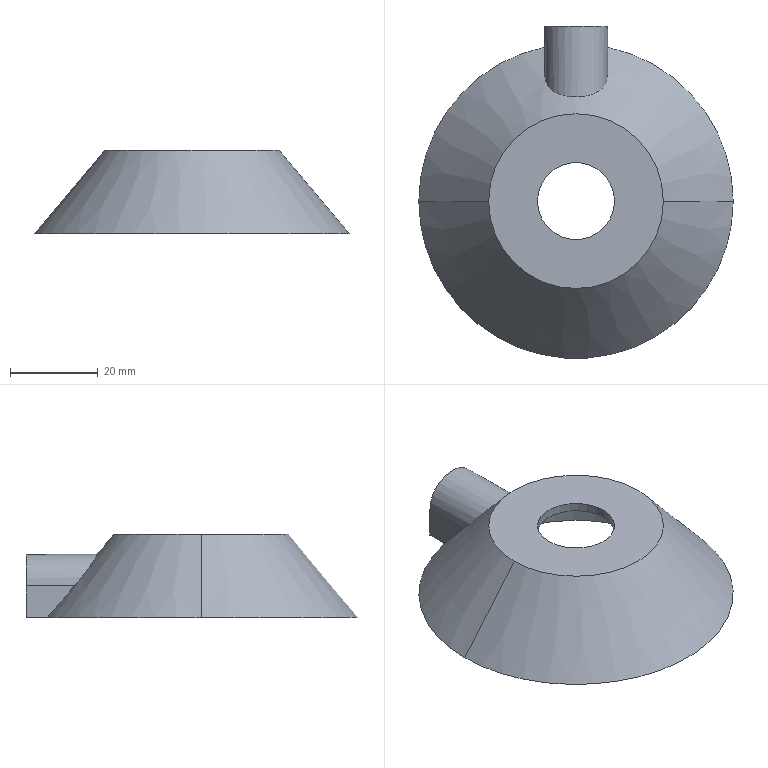Part | SolidWorks | features ICE 5, Extrusion 1, RevCut 1 | 1 solid | 30 faces | box 71.8 x 75.9 x 19 mm | volume 15603 mm3 | plane 12 | cylinder 11 | cone 7 | commonest cylinder face diameters 58 x3 62 x3 5.4 x2 17.6 x2 14.4 x1
STEP:
#1=CARTESIAN_POINT('',(2.7,26.139,6.7));
#2=VERTEX_POINT('',#1);
#3=CARTESIAN_POINT('',(0.,24.012,9.4));
#4=VERTEX_POINT('',#3);
#5=CARTESIAN_POINT('',(2.7,26.139,6.7));
#6=CARTESIAN_POINT('',(2.7,26.009,6.854));
#7=CARTESIAN_POINT('',(2.687,25.881,7.008));
#8=CARTESIAN_POINT('',(2.633,25.626,7.316));
#9=CARTESIAN_POINT('',(2.593,25.5,7.471));
#10=CARTESIAN_POINT('',(2.483,25.256,7.773));
#11=CARTESIAN_POINT('',(2.414,25.138,7.921));
#12=CARTESIAN_POINT('',(2.246,24.912,8.208));
#13=CARTESIAN_POINT('',(2.145,24.802,8.349));
#14=CARTESIAN_POINT('',(1.914,24.599,8.612));
#15=CARTESIAN_POINT('',(1.784,24.506,8.735));
#16=CARTESIAN_POINT('',(1.492,24.338,8.958));
#17=CARTESIAN_POINT('',(1.329,24.264,9.058));
#18=CARTESIAN_POINT('',(0.9814,24.142,9.223));
#19=CARTESIAN_POINT('',(0.7923,24.094,9.289));
#20=CARTESIAN_POINT('',(0.4032,24.029,9.377));
#21=CARTESIAN_POINT('',(0.204,24.012,9.4));
#22=CARTESIAN_POINT('',(0.,24.012,9.4));
#23=B_SPLINE_CURVE_WITH_KNOTS('',3,(#5,#6,#7,#8,#9,#10,#11,#12,#13,#14,#15,#16,#17,#18,#19,#20,#21,#22),.UNSPECIFIED.,.F.,.F.,(4,2,2,2,2,2,2,2,4),(0.0003524,0.0009553,0.001558,0.002161,0.002764,0.003367,0.00397,0.004572,0.005175),.UNSPECIFIED.);
#24=EDGE_CURVE('',#2,#4,#23,.T.);
#25=ORIENTED_EDGE('',*,*,#24,.T.);
#26=CARTESIAN_POINT('',(0.,40.,9.4));
#27=VERTEX_POINT('',#26);
#28=CARTESIAN_POINT('',(0.,24.,9.4));
#29=DIRECTION('',(0.,1.,0.));
#30=VECTOR('',#29,1000.);
#31=LINE('',#28,#30);
#32=EDGE_CURVE('',#4,#27,#31,.T.);
#33=ORIENTED_EDGE('',*,*,#32,.T.);
#34=CARTESIAN_POINT('',(2.7,40.,6.7));
#35=VERTEX_POINT('',#34);
#36=CARTESIAN_POINT('',(0.,40.,6.7));
#37=DIRECTION('',(0.,1.,0.));
#38=DIRECTION('',(0.,0.,1.));
#39=AXIS2_PLACEMENT_3D('',#36,#37,#38);
#40=CIRCLE('',#39,2.7);
#41=EDGE_CURVE('',#27,#35,#40,.T.);
#42=ORIENTED_EDGE('',*,*,#41,.T.);
#43=CARTESIAN_POINT('',(2.7,24.,6.7));
#44=DIRECTION('',(0.,1.,0.));
#45=VECTOR('',#44,1000.);
#46=LINE('',#43,#45);
#47=EDGE_CURVE('',#2,#35,#46,.T.);
#48=ORIENTED_EDGE('',*,*,#47,.F.);
#49=EDGE_LOOP('',(#25,#33,#42,#48));
#50=FACE_OUTER_BOUND('',#49,.T.);
#51=CARTESIAN_POINT('',(0.,24.,6.7));
#52=DIRECTION('',(0.,1.,0.));
#53=DIRECTION('',(0.,0.,1.));
#54=AXIS2_PLACEMENT_3D('',#51,#52,#53);
#55=CYLINDRICAL_SURFACE('',#54,2.7);
#56=ADVANCED_FACE('',(#50),#55,.F.);
#57=CARTESIAN_POINT('',(-8.8,0.,17.));
#58=VERTEX_POINT('',#57);
#59=CARTESIAN_POINT('',(8.8,0.,17.));
#60=VERTEX_POINT('',#59);
#61=CARTESIAN_POINT('',(0.,0.,17.));
#62=DIRECTION('',(0.,0.,1.));
#63=DIRECTION('',(1.,0.,0.));
#64=AXIS2_PLACEMENT_3D('',#61,#62,#63);
#65=CIRCLE('',#64,8.8);
#66=EDGE_CURVE('',#58,#60,#65,.T.);
#67=ORIENTED_EDGE('',*,*,#66,.F.);
#68=CARTESIAN_POINT('',(-8.8,0.,19.));
#69=VERTEX_POINT('',#68);
#70=CARTESIAN_POINT('',(-8.8,0.,17.));
#71=DIRECTION('',(0.,0.,1.));
#72=VECTOR('',#71,1000.);
#73=LINE('',#70,#72);
#74=EDGE_CURVE('',#58,#69,#73,.T.);
#75=ORIENTED_EDGE('',*,*,#74,.T.);
#76=CARTESIAN_POINT('',(8.8,0.,19.));
#77=VERTEX_POINT('',#76);
#78=CARTESIAN_POINT('',(0.,0.,19.));
#79=DIRECTION('',(0.,0.,1.));
#80=DIRECTION('',(1.,0.,0.));
#81=AXIS2_PLACEMENT_3D('',#78,#79,#80);
#82=CIRCLE('',#81,8.8);
#83=EDGE_CURVE('',#69,#77,#82,.T.);
#84=ORIENTED_EDGE('',*,*,#83,.T.);
#85=CARTESIAN_POINT('',(8.8,0.,17.));
#86=DIRECTION('',(0.,0.,1.));
#87=VECTOR('',#86,1000.);
#88=LINE('',#85,#87);
#89=EDGE_CURVE('',#60,#77,#88,.T.);
#90=ORIENTED_EDGE('',*,*,#89,.F.);
#91=EDGE_LOOP('',(#67,#75,#84,#90));
#92=FACE_OUTER_BOUND('',#91,.T.);
#93=CARTESIAN_POINT('',(0.,0.,17.));
#94=DIRECTION('',(0.,0.,1.));
#95=DIRECTION('',(1.,0.,0.));
#96=AXIS2_PLACEMENT_3D('',#93,#94,#95);
#97=CYLINDRICAL_SURFACE('',#96,8.8);
#98=ADVANCED_FACE('',(#92),#97,.F.);
#99=CARTESIAN_POINT('',(17.635,0.,17.));
#100=VERTEX_POINT('',#99);
#101=CARTESIAN_POINT('',(-17.635,0.,17.));
#102=VERTEX_POINT('',#101);
#103=CARTESIAN_POINT('',(0.,0.,17.));
#104=DIRECTION('',(0.,0.,-1.));
#105=DIRECTION('',(-1.,0.,0.));
#106=AXIS2_PLACEMENT_3D('',#103,#104,#105);
#107=CIRCLE('',#106,17.635);
#108=EDGE_CURVE('',#100,#102,#107,.T.);
#109=ORIENTED_EDGE('',*,*,#108,.F.);
#110=CARTESIAN_POINT('',(29.,0.,3.456));
#111=VERTEX_POINT('',#110);
#112=CARTESIAN_POINT('',(17.635,0.,17.));
#113=DIRECTION('',(0.6428,0.,-0.766));
#114=VECTOR('',#113,1000.);
#115=LINE('',#112,#114);
#116=EDGE_CURVE('',#100,#111,#115,.T.);
#117=ORIENTED_EDGE('',*,*,#116,.T.);
#118=CARTESIAN_POINT('',(-29.,0.,3.456));
#119=VERTEX_POINT('',#118);
#120=CARTESIAN_POINT('',(0.,0.,3.456));
#121=DIRECTION('',(0.,0.,1.));
#122=DIRECTION('',(-1.,0.,0.));
#123=AXIS2_PLACEMENT_3D('',#120,#121,#122);
#124=CIRCLE('',#123,29.);
#125=EDGE_CURVE('',#119,#111,#124,.T.);
#126=ORIENTED_EDGE('',*,*,#125,.F.);
#127=CARTESIAN_POINT('',(-17.635,0.,17.));
#128=DIRECTION('',(-0.6428,0.,-0.766));
#129=VECTOR('',#128,1000.);
#130=LINE('',#127,#129);
#131=EDGE_CURVE('',#102,#119,#130,.T.);
#132=ORIENTED_EDGE('',*,*,#131,.F.);
#133=EDGE_LOOP('',(#109,#117,#126,#132));
#134=FACE_OUTER_BOUND('',#133,.T.);
#135=CARTESIAN_POINT('',(0.,0.,17.));
#136=DIRECTION('',(0.,0.,-1.));
#137=DIRECTION('',(-1.,0.,0.));
#138=AXIS2_PLACEMENT_3D('',#135,#136,#137);
#139=CONICAL_SURFACE('',#138,17.635,0.6981);
#140=ADVANCED_FACE('',(#134),#139,.F.);
#141=ORIENTED_EDGE('',*,*,#125,.T.);
#142=CARTESIAN_POINT('',(29.,0.,0.));
#143=VERTEX_POINT('',#142);
#144=CARTESIAN_POINT('',(29.,0.,38.017));
#145=DIRECTION('',(0.,0.,-1.));
#146=VECTOR('',#145,1000.);
#147=LINE('',#144,#146);
#148=EDGE_CURVE('',#111,#143,#147,.T.);
#149=ORIENTED_EDGE('',*,*,#148,.T.);
#150=CARTESIAN_POINT('',(-29.,0.,0.));
#151=VERTEX_POINT('',#150);
#152=CARTESIAN_POINT('',(0.,0.,0.));
#153=DIRECTION('',(0.,0.,-1.));
#154=DIRECTION('',(-1.,0.,0.));
#155=AXIS2_PLACEMENT_3D('',#152,#153,#154);
#156=CIRCLE('',#155,29.);
#157=EDGE_CURVE('',#143,#151,#156,.T.);
#158=ORIENTED_EDGE('',*,*,#157,.T.);
#159=CARTESIAN_POINT('',(-29.,0.,38.017));
#160=DIRECTION('',(0.,0.,-1.));
#161=VECTOR('',#160,1000.);
#162=LINE('',#159,#161);
#163=EDGE_CURVE('',#119,#151,#162,.T.);
#164=ORIENTED_EDGE('',*,*,#163,.F.);
#165=EDGE_LOOP('',(#141,#149,#158,#164));
#166=FACE_OUTER_BOUND('',#165,.T.);
#167=CARTESIAN_POINT('',(0.,0.,38.017));
#168=DIRECTION('',(0.,0.,-1.));
#169=DIRECTION('',(-1.,0.,0.));
#170=AXIS2_PLACEMENT_3D('',#167,#168,#169);
#171=CYLINDRICAL_SURFACE('',#170,29.);
#172=ADVANCED_FACE('',(#166),#171,.F.);
#173=CARTESIAN_POINT('',(-3.7,28.763,3.456));
#174=VERTEX_POINT('',#173);
#175=CARTESIAN_POINT('',(0.,0.,3.456));
#176=DIRECTION('',(0.,0.,1.));
#177=DIRECTION('',(-1.,0.,0.));
#178=AXIS2_PLACEMENT_3D('',#175,#176,#177);
#179=CIRCLE('',#178,29.);
#180=EDGE_CURVE('',#174,#119,#179,.T.);
#181=ORIENTED_EDGE('',*,*,#180,.T.);
#182=ORIENTED_EDGE('',*,*,#163,.T.);
#183=CARTESIAN_POINT('',(-3.7,28.763,0.));
#184=VERTEX_POINT('',#183);
#185=CARTESIAN_POINT('',(0.,0.,0.));
#186=DIRECTION('',(0.,0.,-1.));
#187=DIRECTION('',(-1.,0.,0.));
#188=AXIS2_PLACEMENT_3D('',#185,#186,#187);
#189=CIRCLE('',#188,29.);
#190=EDGE_CURVE('',#151,#184,#189,.T.);
#191=ORIENTED_EDGE('',*,*,#190,.T.);
#192=CARTESIAN_POINT('',(-3.7,28.763,38.017));
#193=DIRECTION('',(0.,0.,1.));
#194=VECTOR('',#193,1000.);
#195=LINE('',#192,#194);
#196=EDGE_CURVE('',#184,#174,#195,.T.);
#197=ORIENTED_EDGE('',*,*,#196,.T.);
#198=EDGE_LOOP('',(#181,#182,#191,#197));
#199=FACE_OUTER_BOUND('',#198,.T.);
#200=CARTESIAN_POINT('',(0.,0.,38.017));
#201=DIRECTION('',(0.,0.,-1.));
#202=DIRECTION('',(-1.,0.,0.));
#203=AXIS2_PLACEMENT_3D('',#200,#201,#202);
#204=CYLINDRICAL_SURFACE('',#203,29.);
#205=ADVANCED_FACE('',(#199),#204,.F.);
#206=CARTESIAN_POINT('',(5.9,30.433,1.073));
#207=VERTEX_POINT('',#206);
#208=CARTESIAN_POINT('',(31.,0.,1.073));
#209=VERTEX_POINT('',#208);
#210=CARTESIAN_POINT('',(0.,0.,1.073));
#211=DIRECTION('',(0.,0.,-1.));
#212=DIRECTION('',(-1.,0.,0.));
#213=AXIS2_PLACEMENT_3D('',#210,#211,#212);
#214=CIRCLE('',#213,31.);
#215=EDGE_CURVE('',#207,#209,#214,.T.);
#216=ORIENTED_EDGE('',*,*,#215,.T.);
#217=CARTESIAN_POINT('',(31.,0.,0.));
#218=VERTEX_POINT('',#217);
#219=CARTESIAN_POINT('',(31.,0.,38.017));
#220=DIRECTION('',(0.,0.,-1.));
#221=VECTOR('',#220,1000.);
#222=LINE('',#219,#221);
#223=EDGE_CURVE('',#209,#218,#222,.T.);
#224=ORIENTED_EDGE('',*,*,#223,.T.);
#225=CARTESIAN_POINT('',(5.9,30.433,0.));
#226=VERTEX_POINT('',#225);
#227=CARTESIAN_POINT('',(0.,0.,0.));
#228=DIRECTION('',(0.,0.,-1.));
#229=DIRECTION('',(-1.,0.,0.));
#230=AXIS2_PLACEMENT_3D('',#227,#228,#229);
#231=CIRCLE('',#230,31.);
#232=EDGE_CURVE('',#226,#218,#231,.T.);
#233=ORIENTED_EDGE('',*,*,#232,.F.);
#234=CARTESIAN_POINT('',(5.9,30.433,38.017));
#235=DIRECTION('',(0.,0.,-1.));
#236=VECTOR('',#235,1000.);
#237=LINE('',#234,#236);
#238=EDGE_CURVE('',#207,#226,#237,.T.);
#239=ORIENTED_EDGE('',*,*,#238,.F.);
#240=EDGE_LOOP('',(#216,#224,#233,#239));
#241=FACE_OUTER_BOUND('',#240,.T.);
#242=CARTESIAN_POINT('',(0.,0.,38.017));
#243=DIRECTION('',(0.,0.,-1.));
#244=DIRECTION('',(-1.,0.,0.));
#245=AXIS2_PLACEMENT_3D('',#242,#243,#244);
#246=CYLINDRICAL_SURFACE('',#245,31.);
#247=ADVANCED_FACE('',(#241),#246,.T.);
#248=ORIENTED_EDGE('',*,*,#223,.F.);
#249=CARTESIAN_POINT('',(-31.,0.,1.073));
#250=VERTEX_POINT('',#249);
#251=CARTESIAN_POINT('',(0.,0.,1.073));
#252=DIRECTION('',(0.,0.,-1.));
#253=DIRECTION('',(-1.,0.,0.));
#254=AXIS2_PLACEMENT_3D('',#251,#252,#253);
#255=CIRCLE('',#254,31.);
#256=EDGE_CURVE('',#209,#250,#255,.T.);
#257=ORIENTED_EDGE('',*,*,#256,.T.);
#258=CARTESIAN_POINT('',(-31.,0.,0.));
#259=VERTEX_POINT('',#258);
#260=CARTESIAN_POINT('',(-31.,0.,38.017));
#261=DIRECTION('',(0.,0.,-1.));
#262=VECTOR('',#261,1000.);
#263=LINE('',#260,#262);
#264=EDGE_CURVE('',#250,#259,#263,.T.);
#265=ORIENTED_EDGE('',*,*,#264,.T.);
#266=CARTESIAN_POINT('',(0.,0.,0.));
#267=DIRECTION('',(0.,0.,-1.));
#268=DIRECTION('',(-1.,0.,0.));
#269=AXIS2_PLACEMENT_3D('',#266,#267,#268);
#270=CIRCLE('',#269,31.);
#271=EDGE_CURVE('',#218,#259,#270,.T.);
#272=ORIENTED_EDGE('',*,*,#271,.F.);
#273=EDGE_LOOP('',(#248,#257,#265,#272));
#274=FACE_OUTER_BOUND('',#273,.T.);
#275=CARTESIAN_POINT('',(0.,0.,38.017));
#276=DIRECTION('',(0.,0.,-1.));
#277=DIRECTION('',(-1.,0.,0.));
#278=AXIS2_PLACEMENT_3D('',#275,#276,#277);
#279=CYLINDRICAL_SURFACE('',#278,31.);
#280=ADVANCED_FACE('',(#274),#279,.T.);
#281=ORIENTED_EDGE('',*,*,#256,.F.);
#282=CARTESIAN_POINT('',(31.9,0.,0.));
#283=VERTEX_POINT('',#282);
#284=CARTESIAN_POINT('',(17.635,0.,17.));
#285=DIRECTION('',(0.6428,0.,-0.766));
#286=VECTOR('',#285,1000.);
#287=LINE('',#284,#286);
#288=EDGE_CURVE('',#209,#283,#287,.T.);
#289=ORIENTED_EDGE('',*,*,#288,.T.);
#290=CARTESIAN_POINT('',(-31.9,0.,0.));
#291=VERTEX_POINT('',#290);
#292=CARTESIAN_POINT('',(0.,0.,0.));
#293=DIRECTION('',(0.,0.,-1.));
#294=DIRECTION('',(-1.,0.,0.));
#295=AXIS2_PLACEMENT_3D('',#292,#293,#294);
#296=CIRCLE('',#295,31.9);
#297=EDGE_CURVE('',#283,#291,#296,.T.);
#298=ORIENTED_EDGE('',*,*,#297,.T.);
#299=CARTESIAN_POINT('',(-17.635,0.,17.));
#300=DIRECTION('',(-0.6428,0.,-0.766));
#301=VECTOR('',#300,1000.);
#302=LINE('',#299,#301);
#303=EDGE_CURVE('',#250,#291,#302,.T.);
#304=ORIENTED_EDGE('',*,*,#303,.F.);
#305=EDGE_LOOP('',(#281,#289,#298,#304));
#306=FACE_OUTER_BOUND('',#305,.T.);
#307=CARTESIAN_POINT('',(0.,0.,17.));
#308=DIRECTION('',(0.,0.,-1.));
#309=DIRECTION('',(-1.,0.,0.));
#310=AXIS2_PLACEMENT_3D('',#307,#308,#309);
#311=CONICAL_SURFACE('',#310,17.635,0.6981);
#312=ADVANCED_FACE('',(#306),#311,.F.);
#313=CARTESIAN_POINT('',(-5.9,30.433,1.073));
#314=VERTEX_POINT('',#313);
#315=CARTESIAN_POINT('',(0.,0.,1.073));
#316=DIRECTION('',(0.,0.,-1.));
#317=DIRECTION('',(-1.,0.,0.));
#318=AXIS2_PLACEMENT_3D('',#315,#316,#317);
#319=CIRCLE('',#318,31.);
#320=EDGE_CURVE('',#250,#314,#319,.T.);
#321=ORIENTED_EDGE('',*,*,#320,.F.);
#322=ORIENTED_EDGE('',*,*,#303,.T.);
#323=CARTESIAN_POINT('',(-5.9,31.35,0.));
#324=VERTEX_POINT('',#323);
#325=CARTESIAN_POINT('',(0.,0.,0.));
#326=DIRECTION('',(0.,0.,-1.));
#327=DIRECTION('',(-1.,0.,0.));
#328=AXIS2_PLACEMENT_3D('',#325,#326,#327);
#329=CIRCLE('',#328,31.9);
#330=EDGE_CURVE('',#291,#324,#329,.T.);
#331=ORIENTED_EDGE('',*,*,#330,.T.);
#332=CARTESIAN_POINT('',(-5.9,30.433,1.073));
#333=CARTESIAN_POINT('',(-5.9,30.739,0.7151));
#334=CARTESIAN_POINT('',(-5.9,31.044,0.3576));
#335=CARTESIAN_POINT('',(-5.9,31.35,0.));
#336=B_SPLINE_CURVE_WITH_KNOTS('',3,(#332,#333,#334,#335),.UNSPECIFIED.,.F.,.F.,(4,4),(0.006323,0.007734),.UNSPECIFIED.);
#337=EDGE_CURVE('',#314,#324,#336,.T.);
#338=ORIENTED_EDGE('',*,*,#337,.F.);
#339=EDGE_LOOP('',(#321,#322,#331,#338));
#340=FACE_OUTER_BOUND('',#339,.T.);
#341=CARTESIAN_POINT('',(0.,0.,17.));
#342=DIRECTION('',(0.,0.,-1.));
#343=DIRECTION('',(-1.,0.,0.));
#344=AXIS2_PLACEMENT_3D('',#341,#342,#343);
#345=CONICAL_SURFACE('',#344,17.635,0.6981);
#346=ADVANCED_FACE('',(#340),#345,.F.);
#347=CARTESIAN_POINT('',(-19.957,0.,19.));
#348=VERTEX_POINT('',#347);
#349=CARTESIAN_POINT('',(19.957,0.,19.));
#350=VERTEX_POINT('',#349);
#351=CARTESIAN_POINT('',(0.,0.,19.));
#352=DIRECTION('',(0.,0.,1.));
#353=DIRECTION('',(1.,0.,0.));
#354=AXIS2_PLACEMENT_3D('',#351,#352,#353);
#355=CIRCLE('',#354,19.957);
#356=EDGE_CURVE('',#348,#350,#355,.T.);
#357=ORIENTED_EDGE('',*,*,#356,.F.);
#358=CARTESIAN_POINT('',(-35.9,0.,0.));
#359=VERTEX_POINT('',#358);
#360=CARTESIAN_POINT('',(-35.9,0.,0.));
#361=DIRECTION('',(-0.6428,0.,-0.766));
#362=VECTOR('',#361,1000.);
#363=LINE('',#360,#362);
#364=EDGE_CURVE('',#348,#359,#363,.T.);
#365=ORIENTED_EDGE('',*,*,#364,.T.);
#366=CARTESIAN_POINT('',(35.9,0.,0.));
#367=VERTEX_POINT('',#366);
#368=CARTESIAN_POINT('',(0.,0.,0.));
#369=DIRECTION('',(0.,0.,1.));
#370=DIRECTION('',(1.,0.,0.));
#371=AXIS2_PLACEMENT_3D('',#368,#369,#370);
#372=CIRCLE('',#371,35.9);
#373=EDGE_CURVE('',#359,#367,#372,.T.);
#374=ORIENTED_EDGE('',*,*,#373,.T.);
#375=CARTESIAN_POINT('',(35.9,0.,0.));
#376=DIRECTION('',(0.6428,0.,-0.766));
#377=VECTOR('',#376,1000.);
#378=LINE('',#375,#377);
#379=EDGE_CURVE('',#350,#367,#378,.T.);
#380=ORIENTED_EDGE('',*,*,#379,.F.);
#381=EDGE_LOOP('',(#357,#365,#374,#380));
#382=FACE_OUTER_BOUND('',#381,.T.);
#383=CARTESIAN_POINT('',(0.,0.,0.));
#384=DIRECTION('',(0.,0.,-1.));
#385=DIRECTION('',(1.,0.,0.));
#386=AXIS2_PLACEMENT_3D('',#383,#384,#385);
#387=CONICAL_SURFACE('',#386,35.9,0.6981);
#388=ADVANCED_FACE('',(#382),#387,.T.);
#389=CARTESIAN_POINT('',(-5.9,30.433,0.));
#390=VERTEX_POINT('',#389);
#391=CARTESIAN_POINT('',(-5.9,-35.901,0.));
#392=DIRECTION('',(0.,1.,0.));
#393=VECTOR('',#392,1000.);
#394=LINE('',#391,#393);
#395=EDGE_CURVE('',#390,#324,#394,.T.);
#396=ORIENTED_EDGE('',*,*,#395,.T.);
#397=ORIENTED_EDGE('',*,*,#330,.F.);
#398=ORIENTED_EDGE('',*,*,#297,.F.);
#399=CARTESIAN_POINT('',(5.9,31.35,0.));
#400=VERTEX_POINT('',#399);
#401=CARTESIAN_POINT('',(0.,0.,0.));
#402=DIRECTION('',(0.,0.,-1.));
#403=DIRECTION('',(-1.,0.,0.));
#404=AXIS2_PLACEMENT_3D('',#401,#402,#403);
#405=CIRCLE('',#404,31.9);
#406=EDGE_CURVE('',#400,#283,#405,.T.);
#407=ORIENTED_EDGE('',*,*,#406,.F.);
#408=CARTESIAN_POINT('',(5.9,-35.901,0.));
#409=DIRECTION('',(0.,1.,0.));
#410=VECTOR('',#409,1000.);
#411=LINE('',#408,#410);
#412=EDGE_CURVE('',#226,#400,#411,.T.);
#413=ORIENTED_EDGE('',*,*,#412,.F.);
#414=ORIENTED_EDGE('',*,*,#232,.T.);
#415=ORIENTED_EDGE('',*,*,#271,.T.);
#416=CARTESIAN_POINT('',(0.,0.,0.));
#417=DIRECTION('',(0.,0.,-1.));
#418=DIRECTION('',(-1.,0.,0.));
#419=AXIS2_PLACEMENT_3D('',#416,#417,#418);
#420=CIRCLE('',#419,31.);
#421=EDGE_CURVE('',#259,#390,#420,.T.);
#422=ORIENTED_EDGE('',*,*,#421,.T.);
#423=EDGE_LOOP('',(#396,#397,#398,#407,#413,#414,#415,#422));
#424=FACE_BOUND('',#423,.T.);
#425=CARTESIAN_POINT('',(-7.2,40.,0.));
#426=VERTEX_POINT('',#425);
#427=CARTESIAN_POINT('',(-7.2,35.171,0.));
#428=VERTEX_POINT('',#427);
#429=CARTESIAN_POINT('',(-7.2,40.,0.));
#430=DIRECTION('',(0.,-1.,0.));
#431=VECTOR('',#430,1000.);
#432=LINE('',#429,#431);
#433=EDGE_CURVE('',#426,#428,#432,.T.);
#434=ORIENTED_EDGE('',*,*,#433,.F.);
#435=CARTESIAN_POINT('',(-3.7,40.,0.));
#436=VERTEX_POINT('',#435);
#437=CARTESIAN_POINT('',(-7.2,40.,0.));
#438=DIRECTION('',(-1.,0.,0.));
#439=VECTOR('',#438,1000.);
#440=LINE('',#437,#439);
#441=EDGE_CURVE('',#436,#426,#440,.T.);
#442=ORIENTED_EDGE('',*,*,#441,.F.);
#443=CARTESIAN_POINT('',(-3.7,24.,0.));
#444=DIRECTION('',(0.,1.,0.));
#445=VECTOR('',#444,1000.);
#446=LINE('',#443,#445);
#447=EDGE_CURVE('',#184,#436,#446,.T.);
#448=ORIENTED_EDGE('',*,*,#447,.F.);
#449=ORIENTED_EDGE('',*,*,#190,.F.);
#450=ORIENTED_EDGE('',*,*,#157,.F.);
#451=CARTESIAN_POINT('',(3.7,28.763,0.));
#452=VERTEX_POINT('',#451);
#453=CARTESIAN_POINT('',(0.,0.,0.));
#454=DIRECTION('',(0.,0.,-1.));
#455=DIRECTION('',(-1.,0.,0.));
#456=AXIS2_PLACEMENT_3D('',#453,#454,#455);
#457=CIRCLE('',#456,29.);
#458=EDGE_CURVE('',#452,#143,#457,.T.);
#459=ORIENTED_EDGE('',*,*,#458,.F.);
#460=CARTESIAN_POINT('',(3.7,40.,0.));
#461=VERTEX_POINT('',#460);
#462=CARTESIAN_POINT('',(3.7,24.,0.));
#463=DIRECTION('',(0.,1.,0.));
#464=VECTOR('',#463,1000.);
#465=LINE('',#462,#464);
#466=EDGE_CURVE('',#452,#461,#465,.T.);
#467=ORIENTED_EDGE('',*,*,#466,.T.);
#468=CARTESIAN_POINT('',(7.2,40.,0.));
#469=VERTEX_POINT('',#468);
#470=CARTESIAN_POINT('',(-7.2,40.,0.));
#471=DIRECTION('',(-1.,0.,0.));
#472=VECTOR('',#471,1000.);
#473=LINE('',#470,#472);
#474=EDGE_CURVE('',#469,#461,#473,.T.);
#475=ORIENTED_EDGE('',*,*,#474,.F.);
#476=CARTESIAN_POINT('',(7.2,35.171,0.));
#477=VERTEX_POINT('',#476);
#478=CARTESIAN_POINT('',(7.2,40.,0.));
#479=DIRECTION('',(0.,-1.,0.));
#480=VECTOR('',#479,1000.);
#481=LINE('',#478,#480);
#482=EDGE_CURVE('',#469,#477,#481,.T.);
#483=ORIENTED_EDGE('',*,*,#482,.T.);
#484=CARTESIAN_POINT('',(0.,0.,0.));
#485=DIRECTION('',(0.,0.,1.));
#486=DIRECTION('',(1.,0.,0.));
#487=AXIS2_PLACEMENT_3D('',#484,#485,#486);
#488=CIRCLE('',#487,35.9);
#489=EDGE_CURVE('',#367,#477,#488,.T.);
#490=ORIENTED_EDGE('',*,*,#489,.F.);
#491=ORIENTED_EDGE('',*,*,#373,.F.);
#492=CARTESIAN_POINT('',(0.,0.,0.));
#493=DIRECTION('',(0.,0.,1.));
#494=DIRECTION('',(1.,0.,0.));
#495=AXIS2_PLACEMENT_3D('',#492,#493,#494);
#496=CIRCLE('',#495,35.9);
#497=EDGE_CURVE('',#428,#359,#496,.T.);
#498=ORIENTED_EDGE('',*,*,#497,.F.);
#499=EDGE_LOOP('',(#434,#442,#448,#449,#450,#459,#467,#475,#483,#490,#491,#498));
#500=FACE_OUTER_BOUND('',#499,.T.);
#501=CARTESIAN_POINT('',(0.,0.,0.));
#502=DIRECTION('',(0.,0.,1.));
#503=DIRECTION('',(1.,0.,0.));
#504=AXIS2_PLACEMENT_3D('',#501,#502,#503);
#505=PLANE('',#504);
#506=ADVANCED_FACE('',(#424,#500),#505,.F.);
#507=ORIENTED_EDGE('',*,*,#364,.F.);
#508=CARTESIAN_POINT('',(0.,0.,19.));
#509=DIRECTION('',(0.,0.,1.));
#510=DIRECTION('',(1.,0.,0.));
#511=AXIS2_PLACEMENT_3D('',#508,#509,#510);
#512=CIRCLE('',#511,19.957);
#513=EDGE_CURVE('',#350,#348,#512,.T.);
#514=ORIENTED_EDGE('',*,*,#513,.F.);
#515=ORIENTED_EDGE('',*,*,#379,.T.);
#516=ORIENTED_EDGE('',*,*,#489,.T.);
#517=CARTESIAN_POINT('',(7.2,28.934,7.25));
#518=VERTEX_POINT('',#517);
#519=CARTESIAN_POINT('',(7.2,28.934,7.25));
#520=CARTESIAN_POINT('',(7.2,31.019,4.839));
#521=CARTESIAN_POINT('',(7.2,33.097,2.421));
#522=CARTESIAN_POINT('',(7.2,35.171,0.));
#523=B_SPLINE_CURVE_WITH_KNOTS('',3,(#519,#520,#521,#522),.UNSPECIFIED.,.F.,.F.,(4,4),(0.03537,0.04491),.UNSPECIFIED.);
#524=EDGE_CURVE('',#518,#477,#523,.T.);
#525=ORIENTED_EDGE('',*,*,#524,.F.);
#526=CARTESIAN_POINT('',(-7.2,28.934,7.25));
#527=VERTEX_POINT('',#526);
#528=CARTESIAN_POINT('',(-7.2,28.934,7.25));
#529=CARTESIAN_POINT('',(-7.2,28.588,7.65));
#530=CARTESIAN_POINT('',(-7.167,28.249,8.052));
#531=CARTESIAN_POINT('',(-7.064,27.75,8.658));
#532=CARTESIAN_POINT('',(-7.021,27.585,8.861));
#533=CARTESIAN_POINT('',(-6.915,27.26,9.268));
#534=CARTESIAN_POINT('',(-6.852,27.099,9.473));
#535=CARTESIAN_POINT('',(-6.635,26.629,10.078));
#536=CARTESIAN_POINT('',(-6.453,26.332,10.475));
#537=CARTESIAN_POINT('',(-6.116,25.911,11.056));
#538=CARTESIAN_POINT('',(-5.993,25.775,11.247));
#539=CARTESIAN_POINT('',(-5.723,25.512,11.625));
#540=CARTESIAN_POINT('',(-5.577,25.385,11.81));
#541=CARTESIAN_POINT('',(-5.11,25.027,12.344));
#542=CARTESIAN_POINT('',(-4.758,24.814,12.677));
#543=CARTESIAN_POINT('',(-4.163,24.533,13.13));
#544=CARTESIAN_POINT('',(-3.953,24.446,13.273));
#545=CARTESIAN_POINT('',(-3.52,24.289,13.536));
#546=CARTESIAN_POINT('',(-3.296,24.219,13.656));
#547=CARTESIAN_POINT('',(-2.833,24.093,13.874));
#548=CARTESIAN_POINT('',(-2.594,24.038,13.972));
#549=CARTESIAN_POINT('',(-2.1,23.943,14.142));
#550=CARTESIAN_POINT('',(-1.843,23.902,14.215));
#551=CARTESIAN_POINT('',(-1.071,23.807,14.389));
#552=CARTESIAN_POINT('',(-0.5467,23.776,14.449));
#553=CARTESIAN_POINT('',(0.2534,23.775,14.45));
#554=CARTESIAN_POINT('',(0.5221,23.783,14.436));
#555=CARTESIAN_POINT('',(1.049,23.814,14.378));
#556=CARTESIAN_POINT('',(1.309,23.837,14.335));
#557=CARTESIAN_POINT('',(2.079,23.931,14.163));
#558=CARTESIAN_POINT('',(2.583,24.026,13.99));
#559=CARTESIAN_POINT('',(3.283,24.215,13.663));
#560=CARTESIAN_POINT('',(3.508,24.285,13.543));
#561=CARTESIAN_POINT('',(3.942,24.441,13.28));
#562=CARTESIAN_POINT('',(4.153,24.528,13.137));
#563=CARTESIAN_POINT('',(4.75,24.809,12.684));
#564=CARTESIAN_POINT('',(5.103,25.022,12.352));
#565=CARTESIAN_POINT('',(5.573,25.382,11.815));
#566=CARTESIAN_POINT('',(5.72,25.509,11.629));
#567=CARTESIAN_POINT('',(5.989,25.771,11.253));
#568=CARTESIAN_POINT('',(6.113,25.907,11.061));
#569=CARTESIAN_POINT('',(6.338,26.188,10.673));
#570=CARTESIAN_POINT('',(6.441,26.334,10.476));
#571=CARTESIAN_POINT('',(6.625,26.633,10.077));
#572=CARTESIAN_POINT('',(6.708,26.787,9.874));
#573=CARTESIAN_POINT('',(7.07,27.573,8.862));
#574=CARTESIAN_POINT('',(7.2,28.238,8.055));
#575=CARTESIAN_POINT('',(7.2,28.934,7.25));
#576=B_SPLINE_CURVE_WITH_KNOTS('',3,(#528,#529,#530,#531,#532,#533,#534,#535,#536,#537,#538,#539,#540,#541,#542,#543,#544,#545,#546,#547,#548,#549,#550,#551,#552,#553,#554,#555,#556,#557,#558,#559,#560,#561,#562,#563,#564,#565,#566,#567,#568,#569,#570,#571,#572,#573,#574,#575),.UNSPECIFIED.,.F.,.F.,(4,2,2,2,2,2,2,2,2,2,2,2,2,2,2,2,2,2,2,2,2,2,2,4),(0.0009523,0.002534,0.003325,0.004116,0.005697,0.006488,0.007279,0.008861,0.009652,0.01044,0.01123,0.01202,0.01361,0.0144,0.01519,0.01677,0.01756,0.01835,0.01993,0.02072,0.02151,0.02231,0.0231,0.02626),.UNSPECIFIED.);
#577=EDGE_CURVE('',#527,#518,#576,.T.);
#578=ORIENTED_EDGE('',*,*,#577,.F.);
#579=CARTESIAN_POINT('',(-7.2,35.171,0.));
#580=CARTESIAN_POINT('',(-7.2,33.097,2.421));
#581=CARTESIAN_POINT('',(-7.2,31.019,4.839));
#582=CARTESIAN_POINT('',(-7.2,28.934,7.25));
#583=B_SPLINE_CURVE_WITH_KNOTS('',3,(#579,#580,#581,#582),.UNSPECIFIED.,.F.,.F.,(4,4),(0.03448,0.04404),.UNSPECIFIED.);
#584=EDGE_CURVE('',#428,#527,#583,.T.);
#585=ORIENTED_EDGE('',*,*,#584,.F.);
#586=ORIENTED_EDGE('',*,*,#497,.T.);
#587=EDGE_LOOP('',(#507,#514,#515,#516,#525,#578,#585,#586));
#588=FACE_OUTER_BOUND('',#587,.T.);
#589=CARTESIAN_POINT('',(0.,0.,0.));
#590=DIRECTION('',(0.,0.,-1.));
#591=DIRECTION('',(1.,0.,0.));
#592=AXIS2_PLACEMENT_3D('',#589,#590,#591);
#593=CONICAL_SURFACE('',#592,35.9,0.6981);
#594=ADVANCED_FACE('',(#588),#593,.T.);
#595=CARTESIAN_POINT('',(0.,0.,19.));
#596=DIRECTION('',(0.,0.,1.));
#597=DIRECTION('',(1.,0.,0.));
#598=AXIS2_PLACEMENT_3D('',#595,#596,#597);
#599=CIRCLE('',#598,8.8);
#600=EDGE_CURVE('',#77,#69,#599,.T.);
#601=ORIENTED_EDGE('',*,*,#600,.F.);
#602=ORIENTED_EDGE('',*,*,#83,.F.);
#603=EDGE_LOOP('',(#601,#602));
#604=FACE_BOUND('',#603,.T.);
#605=ORIENTED_EDGE('',*,*,#513,.T.);
#606=ORIENTED_EDGE('',*,*,#356,.T.);
#607=EDGE_LOOP('',(#605,#606));
#608=FACE_OUTER_BOUND('',#607,.T.);
#609=CARTESIAN_POINT('',(0.,0.,19.));
#610=DIRECTION('',(0.,0.,1.));
#611=DIRECTION('',(1.,0.,0.));
#612=AXIS2_PLACEMENT_3D('',#609,#610,#611);
#613=PLANE('',#612);
#614=ADVANCED_FACE('',(#604,#608),#613,.T.);
#615=CARTESIAN_POINT('',(-7.2,40.,7.25));
#616=VERTEX_POINT('',#615);
#617=CARTESIAN_POINT('',(-7.2,40.,7.25));
#618=DIRECTION('',(0.,-1.,0.));
#619=VECTOR('',#618,1000.);
#620=LINE('',#617,#619);
#621=EDGE_CURVE('',#616,#527,#620,.T.);
#622=ORIENTED_EDGE('',*,*,#621,.T.);
#623=ORIENTED_EDGE('',*,*,#577,.T.);
#624=CARTESIAN_POINT('',(7.2,40.,7.25));
#625=VERTEX_POINT('',#624);
#626=CARTESIAN_POINT('',(7.2,40.,7.25));
#627=DIRECTION('',(0.,-1.,0.));
#628=VECTOR('',#627,1000.);
#629=LINE('',#626,#628);
#630=EDGE_CURVE('',#625,#518,#629,.T.);
#631=ORIENTED_EDGE('',*,*,#630,.F.);
#632=CARTESIAN_POINT('',(0.,40.,7.25));
#633=DIRECTION('',(0.,1.,0.));
#634=DIRECTION('',(0.,0.,1.));
#635=AXIS2_PLACEMENT_3D('',#632,#633,#634);
#636=CIRCLE('',#635,7.2);
#637=EDGE_CURVE('',#616,#625,#636,.T.);
#638=ORIENTED_EDGE('',*,*,#637,.F.);
#639=EDGE_LOOP('',(#622,#623,#631,#638));
#640=FACE_OUTER_BOUND('',#639,.T.);
#641=CARTESIAN_POINT('',(0.,40.,7.25));
#642=DIRECTION('',(0.,-1.,0.));
#643=DIRECTION('',(0.,0.,-1.));
#644=AXIS2_PLACEMENT_3D('',#641,#642,#643);
#645=CYLINDRICAL_SURFACE('',#644,7.2);
#646=ADVANCED_FACE('',(#640),#645,.T.);
#647=ORIENTED_EDGE('',*,*,#433,.T.);
#648=ORIENTED_EDGE('',*,*,#584,.T.);
#649=ORIENTED_EDGE('',*,*,#621,.F.);
#650=CARTESIAN_POINT('',(-7.2,40.,0.));
#651=DIRECTION('',(0.,0.,1.));
#652=VECTOR('',#651,1000.);
#653=LINE('',#650,#652);
#654=EDGE_CURVE('',#426,#616,#653,.T.);
#655=ORIENTED_EDGE('',*,*,#654,.F.);
#656=EDGE_LOOP('',(#647,#648,#649,#655));
#657=FACE_OUTER_BOUND('',#656,.T.);
#658=CARTESIAN_POINT('',(-7.2,40.,0.));
#659=DIRECTION('',(1.,0.,0.));
#660=DIRECTION('',(0.,0.,-1.));
#661=AXIS2_PLACEMENT_3D('',#658,#659,#660);
#662=PLANE('',#661);
#663=ADVANCED_FACE('',(#657),#662,.F.);
#664=ORIENTED_EDGE('',*,*,#630,.T.);
#665=ORIENTED_EDGE('',*,*,#524,.T.);
#666=ORIENTED_EDGE('',*,*,#482,.F.);
#667=CARTESIAN_POINT('',(7.2,40.,0.));
#668=DIRECTION('',(0.,0.,-1.));
#669=VECTOR('',#668,1000.);
#670=LINE('',#667,#669);
#671=EDGE_CURVE('',#625,#469,#670,.T.);
#672=ORIENTED_EDGE('',*,*,#671,.F.);
#673=EDGE_LOOP('',(#664,#665,#666,#672));
#674=FACE_OUTER_BOUND('',#673,.T.);
#675=CARTESIAN_POINT('',(7.2,40.,0.));
#676=DIRECTION('',(-1.,0.,0.));
#677=DIRECTION('',(0.,0.,1.));
#678=AXIS2_PLACEMENT_3D('',#675,#676,#677);
#679=PLANE('',#678);
#680=ADVANCED_FACE('',(#674),#679,.F.);
#681=CARTESIAN_POINT('',(-3.7,40.,6.7));
#682=VERTEX_POINT('',#681);
#683=CARTESIAN_POINT('',(-2.7,40.,6.7));
#684=VERTEX_POINT('',#683);
#685=CARTESIAN_POINT('',(-3.7,40.,6.7));
#686=DIRECTION('',(1.,0.,0.));
#687=VECTOR('',#686,1000.);
#688=LINE('',#685,#687);
#689=EDGE_CURVE('',#682,#684,#688,.T.);
#690=ORIENTED_EDGE('',*,*,#689,.F.);
#691=CARTESIAN_POINT('',(-3.7,40.,0.));
#692=DIRECTION('',(0.,0.,1.));
#693=VECTOR('',#692,1000.);
#694=LINE('',#691,#693);
#695=EDGE_CURVE('',#436,#682,#694,.T.);
#696=ORIENTED_EDGE('',*,*,#695,.F.);
#697=ORIENTED_EDGE('',*,*,#441,.T.);
#698=ORIENTED_EDGE('',*,*,#654,.T.);
#699=ORIENTED_EDGE('',*,*,#637,.T.);
#700=ORIENTED_EDGE('',*,*,#671,.T.);
#701=ORIENTED_EDGE('',*,*,#474,.T.);
#702=CARTESIAN_POINT('',(3.7,40.,6.7));
#703=VERTEX_POINT('',#702);
#704=CARTESIAN_POINT('',(3.7,40.,0.));
#705=DIRECTION('',(0.,0.,-1.));
#706=VECTOR('',#705,1000.);
#707=LINE('',#704,#706);
#708=EDGE_CURVE('',#703,#461,#707,.T.);
#709=ORIENTED_EDGE('',*,*,#708,.F.);
#710=CARTESIAN_POINT('',(3.7,40.,6.7));
#711=DIRECTION('',(1.,0.,0.));
#712=VECTOR('',#711,1000.);
#713=LINE('',#710,#712);
#714=EDGE_CURVE('',#35,#703,#713,.T.);
#715=ORIENTED_EDGE('',*,*,#714,.F.);
#716=ORIENTED_EDGE('',*,*,#41,.F.);
#717=CARTESIAN_POINT('',(0.,40.,6.7));
#718=DIRECTION('',(0.,1.,0.));
#719=DIRECTION('',(0.,0.,1.));
#720=AXIS2_PLACEMENT_3D('',#717,#718,#719);
#721=CIRCLE('',#720,2.7);
#722=EDGE_CURVE('',#684,#27,#721,.T.);
#723=ORIENTED_EDGE('',*,*,#722,.F.);
#724=EDGE_LOOP('',(#690,#696,#697,#698,#699,#700,#701,#709,#715,#716,#723));
#725=FACE_OUTER_BOUND('',#724,.T.);
#726=CARTESIAN_POINT('',(0.,40.,7.25));
#727=DIRECTION('',(0.,1.,0.));
#728=DIRECTION('',(0.,0.,1.));
#729=AXIS2_PLACEMENT_3D('',#726,#727,#728);
#730=PLANE('',#729);
#731=ADVANCED_FACE('',(#725),#730,.T.);
#732=ORIENTED_EDGE('',*,*,#288,.F.);
#733=ORIENTED_EDGE('',*,*,#215,.F.);
#734=CARTESIAN_POINT('',(5.9,31.35,0.));
#735=CARTESIAN_POINT('',(5.9,31.044,0.3576));
#736=CARTESIAN_POINT('',(5.9,30.739,0.7151));
#737=CARTESIAN_POINT('',(5.9,30.433,1.073));
#738=B_SPLINE_CURVE_WITH_KNOTS('',3,(#734,#735,#736,#737),.UNSPECIFIED.,.F.,.F.,(4,4),(0.00575,0.00716),.UNSPECIFIED.);
#739=EDGE_CURVE('',#400,#207,#738,.T.);
#740=ORIENTED_EDGE('',*,*,#739,.F.);
#741=ORIENTED_EDGE('',*,*,#406,.T.);
#742=EDGE_LOOP('',(#732,#733,#740,#741));
#743=FACE_OUTER_BOUND('',#742,.T.);
#744=CARTESIAN_POINT('',(0.,0.,17.));
#745=DIRECTION('',(0.,0.,-1.));
#746=DIRECTION('',(-1.,0.,0.));
#747=AXIS2_PLACEMENT_3D('',#744,#745,#746);
#748=CONICAL_SURFACE('',#747,17.635,0.6981);
#749=ADVANCED_FACE('',(#743),#748,.F.);
#750=ORIENTED_EDGE('',*,*,#264,.F.);
#751=ORIENTED_EDGE('',*,*,#320,.T.);
#752=CARTESIAN_POINT('',(-5.9,30.433,38.017));
#753=DIRECTION('',(0.,0.,1.));
#754=VECTOR('',#753,1000.);
#755=LINE('',#752,#754);
#756=EDGE_CURVE('',#390,#314,#755,.T.);
#757=ORIENTED_EDGE('',*,*,#756,.F.);
#758=ORIENTED_EDGE('',*,*,#421,.F.);
#759=EDGE_LOOP('',(#750,#751,#757,#758));
#760=FACE_OUTER_BOUND('',#759,.T.);
#761=CARTESIAN_POINT('',(0.,0.,38.017));
#762=DIRECTION('',(0.,0.,-1.));
#763=DIRECTION('',(-1.,0.,0.));
#764=AXIS2_PLACEMENT_3D('',#761,#762,#763);
#765=CYLINDRICAL_SURFACE('',#764,31.);
#766=ADVANCED_FACE('',(#760),#765,.T.);
#767=ORIENTED_EDGE('',*,*,#148,.F.);
#768=CARTESIAN_POINT('',(3.7,28.763,3.456));
#769=VERTEX_POINT('',#768);
#770=CARTESIAN_POINT('',(0.,0.,3.456));
#771=DIRECTION('',(0.,0.,1.));
#772=DIRECTION('',(-1.,0.,0.));
#773=AXIS2_PLACEMENT_3D('',#770,#771,#772);
#774=CIRCLE('',#773,29.);
#775=EDGE_CURVE('',#111,#769,#774,.T.);
#776=ORIENTED_EDGE('',*,*,#775,.T.);
#777=CARTESIAN_POINT('',(3.7,28.763,38.017));
#778=DIRECTION('',(0.,0.,-1.));
#779=VECTOR('',#778,1000.);
#780=LINE('',#777,#779);
#781=EDGE_CURVE('',#769,#452,#780,.T.);
#782=ORIENTED_EDGE('',*,*,#781,.T.);
#783=ORIENTED_EDGE('',*,*,#458,.T.);
#784=EDGE_LOOP('',(#767,#776,#782,#783));
#785=FACE_OUTER_BOUND('',#784,.T.);
#786=CARTESIAN_POINT('',(0.,0.,38.017));
#787=DIRECTION('',(0.,0.,-1.));
#788=DIRECTION('',(-1.,0.,0.));
#789=AXIS2_PLACEMENT_3D('',#786,#787,#788);
#790=CYLINDRICAL_SURFACE('',#789,29.);
#791=ADVANCED_FACE('',(#785),#790,.F.);
#792=CARTESIAN_POINT('',(0.,0.,17.));
#793=DIRECTION('',(0.,0.,1.));
#794=DIRECTION('',(1.,0.,0.));
#795=AXIS2_PLACEMENT_3D('',#792,#793,#794);
#796=CIRCLE('',#795,8.8);
#797=EDGE_CURVE('',#60,#58,#796,.T.);
#798=ORIENTED_EDGE('',*,*,#797,.T.);
#799=ORIENTED_EDGE('',*,*,#66,.T.);
#800=EDGE_LOOP('',(#798,#799));
#801=FACE_BOUND('',#800,.T.);
#802=CARTESIAN_POINT('',(0.,0.,17.));
#803=DIRECTION('',(0.,0.,-1.));
#804=DIRECTION('',(-1.,0.,0.));
#805=AXIS2_PLACEMENT_3D('',#802,#803,#804);
#806=CIRCLE('',#805,17.635);
#807=EDGE_CURVE('',#102,#100,#806,.T.);
#808=ORIENTED_EDGE('',*,*,#807,.T.);
#809=ORIENTED_EDGE('',*,*,#108,.T.);
#810=EDGE_LOOP('',(#808,#809));
#811=FACE_OUTER_BOUND('',#810,.T.);
#812=CARTESIAN_POINT('',(0.,0.,17.));
#813=DIRECTION('',(0.,0.,-1.));
#814=DIRECTION('',(-1.,0.,0.));
#815=AXIS2_PLACEMENT_3D('',#812,#813,#814);
#816=PLANE('',#815);
#817=ADVANCED_FACE('',(#801,#811),#816,.T.);
#818=ORIENTED_EDGE('',*,*,#116,.F.);
#819=ORIENTED_EDGE('',*,*,#807,.F.);
#820=ORIENTED_EDGE('',*,*,#131,.T.);
#821=ORIENTED_EDGE('',*,*,#180,.F.);
#822=CARTESIAN_POINT('',(-3.7,26.016,6.7));
#823=VERTEX_POINT('',#822);
#824=CARTESIAN_POINT('',(-3.7,26.016,6.7));
#825=CARTESIAN_POINT('',(-3.7,26.932,5.619));
#826=CARTESIAN_POINT('',(-3.7,27.848,4.538));
#827=CARTESIAN_POINT('',(-3.7,28.763,3.456));
#828=B_SPLINE_CURVE_WITH_KNOTS('',3,(#824,#825,#826,#827),.UNSPECIFIED.,.F.,.F.,(4,4),(0.01103,0.01528),.UNSPECIFIED.);
#829=EDGE_CURVE('',#823,#174,#828,.T.);
#830=ORIENTED_EDGE('',*,*,#829,.F.);
#831=CARTESIAN_POINT('',(-2.7,26.139,6.7));
#832=VERTEX_POINT('',#831);
#833=CARTESIAN_POINT('',(0.,0.,6.7));
#834=DIRECTION('',(0.,0.,1.));
#835=DIRECTION('',(1.,0.,0.));
#836=AXIS2_PLACEMENT_3D('',#833,#834,#835);
#837=CIRCLE('',#836,26.278);
#838=EDGE_CURVE('',#832,#823,#837,.T.);
#839=ORIENTED_EDGE('',*,*,#838,.F.);
#840=CARTESIAN_POINT('',(0.,24.012,9.4));
#841=CARTESIAN_POINT('',(-0.2036,24.012,9.4));
#842=CARTESIAN_POINT('',(-0.4041,24.029,9.377));
#843=CARTESIAN_POINT('',(-0.793,24.094,9.289));
#844=CARTESIAN_POINT('',(-0.9815,24.142,9.223));
#845=CARTESIAN_POINT('',(-1.329,24.264,9.058));
#846=CARTESIAN_POINT('',(-1.492,24.338,8.958));
#847=CARTESIAN_POINT('',(-1.784,24.506,8.735));
#848=CARTESIAN_POINT('',(-1.915,24.6,8.611));
#849=CARTESIAN_POINT('',(-2.262,24.905,8.215));
#850=CARTESIAN_POINT('',(-2.427,25.133,7.926));
#851=CARTESIAN_POINT('',(-2.648,25.622,7.319));
#852=CARTESIAN_POINT('',(-2.7,25.877,7.01));
#853=CARTESIAN_POINT('',(-2.7,26.139,6.7));
#854=B_SPLINE_CURVE_WITH_KNOTS('',3,(#840,#841,#842,#843,#844,#845,#846,#847,#848,#849,#850,#851,#852,#853),.UNSPECIFIED.,.F.,.F.,(4,2,2,2,2,2,4),(0.005175,0.005777,0.006378,0.00698,0.007581,0.008784,0.009987),.UNSPECIFIED.);
#855=EDGE_CURVE('',#4,#832,#854,.T.);
#856=ORIENTED_EDGE('',*,*,#855,.F.);
#857=ORIENTED_EDGE('',*,*,#24,.F.);
#858=CARTESIAN_POINT('',(3.7,26.016,6.7));
#859=VERTEX_POINT('',#858);
#860=CARTESIAN_POINT('',(0.,0.,6.7));
#861=DIRECTION('',(0.,0.,1.));
#862=DIRECTION('',(1.,0.,0.));
#863=AXIS2_PLACEMENT_3D('',#860,#861,#862);
#864=CIRCLE('',#863,26.278);
#865=EDGE_CURVE('',#859,#2,#864,.T.);
#866=ORIENTED_EDGE('',*,*,#865,.F.);
#867=CARTESIAN_POINT('',(3.7,28.763,3.456));
#868=CARTESIAN_POINT('',(3.7,27.848,4.538));
#869=CARTESIAN_POINT('',(3.7,26.932,5.619));
#870=CARTESIAN_POINT('',(3.7,26.016,6.7));
#871=B_SPLINE_CURVE_WITH_KNOTS('',3,(#867,#868,#869,#870),.UNSPECIFIED.,.F.,.F.,(4,4),(0.00783,0.01208),.UNSPECIFIED.);
#872=EDGE_CURVE('',#769,#859,#871,.T.);
#873=ORIENTED_EDGE('',*,*,#872,.F.);
#874=ORIENTED_EDGE('',*,*,#775,.F.);
#875=EDGE_LOOP('',(#818,#819,#820,#821,#830,#839,#856,#857,#866,#873,#874));
#876=FACE_OUTER_BOUND('',#875,.T.);
#877=CARTESIAN_POINT('',(0.,0.,17.));
#878=DIRECTION('',(0.,0.,-1.));
#879=DIRECTION('',(-1.,0.,0.));
#880=AXIS2_PLACEMENT_3D('',#877,#878,#879);
#881=CONICAL_SURFACE('',#880,17.635,0.6981);
#882=ADVANCED_FACE('',(#876),#881,.F.);
#883=ORIENTED_EDGE('',*,*,#74,.F.);
#884=ORIENTED_EDGE('',*,*,#797,.F.);
#885=ORIENTED_EDGE('',*,*,#89,.T.);
#886=ORIENTED_EDGE('',*,*,#600,.T.);
#887=EDGE_LOOP('',(#883,#884,#885,#886));
#888=FACE_OUTER_BOUND('',#887,.T.);
#889=CARTESIAN_POINT('',(0.,0.,17.));
#890=DIRECTION('',(0.,0.,1.));
#891=DIRECTION('',(1.,0.,0.));
#892=AXIS2_PLACEMENT_3D('',#889,#890,#891);
#893=CYLINDRICAL_SURFACE('',#892,8.8);
#894=ADVANCED_FACE('',(#888),#893,.F.);
#895=ORIENTED_EDGE('',*,*,#781,.F.);
#896=ORIENTED_EDGE('',*,*,#872,.T.);
#897=CARTESIAN_POINT('',(3.7,24.,6.7));
#898=DIRECTION('',(0.,1.,0.));
#899=VECTOR('',#898,1000.);
#900=LINE('',#897,#899);
#901=EDGE_CURVE('',#859,#703,#900,.T.);
#902=ORIENTED_EDGE('',*,*,#901,.T.);
#903=ORIENTED_EDGE('',*,*,#708,.T.);
#904=ORIENTED_EDGE('',*,*,#466,.F.);
#905=EDGE_LOOP('',(#895,#896,#902,#903,#904));
#906=FACE_OUTER_BOUND('',#905,.T.);
#907=CARTESIAN_POINT('',(3.7,24.,0.));
#908=DIRECTION('',(1.,0.,0.));
#909=DIRECTION('',(0.,0.,-1.));
#910=AXIS2_PLACEMENT_3D('',#907,#908,#909);
#911=PLANE('',#910);
#912=ADVANCED_FACE('',(#906),#911,.F.);
#913=ORIENTED_EDGE('',*,*,#196,.F.);
#914=ORIENTED_EDGE('',*,*,#447,.T.);
#915=ORIENTED_EDGE('',*,*,#695,.T.);
#916=CARTESIAN_POINT('',(-3.7,24.,6.7));
#917=DIRECTION('',(0.,1.,0.));
#918=VECTOR('',#917,1000.);
#919=LINE('',#916,#918);
#920=EDGE_CURVE('',#823,#682,#919,.T.);
#921=ORIENTED_EDGE('',*,*,#920,.F.);
#922=ORIENTED_EDGE('',*,*,#829,.T.);
#923=EDGE_LOOP('',(#913,#914,#915,#921,#922));
#924=FACE_OUTER_BOUND('',#923,.T.);
#925=CARTESIAN_POINT('',(-3.7,24.,0.));
#926=DIRECTION('',(-1.,0.,0.));
#927=DIRECTION('',(0.,0.,1.));
#928=AXIS2_PLACEMENT_3D('',#925,#926,#927);
#929=PLANE('',#928);
#930=ADVANCED_FACE('',(#924),#929,.F.);
#931=ORIENTED_EDGE('',*,*,#865,.T.);
#932=ORIENTED_EDGE('',*,*,#47,.T.);
#933=ORIENTED_EDGE('',*,*,#714,.T.);
#934=ORIENTED_EDGE('',*,*,#901,.F.);
#935=EDGE_LOOP('',(#931,#932,#933,#934));
#936=FACE_OUTER_BOUND('',#935,.T.);
#937=CARTESIAN_POINT('',(3.7,24.,6.7));
#938=DIRECTION('',(0.,0.,1.));
#939=DIRECTION('',(1.,0.,0.));
#940=AXIS2_PLACEMENT_3D('',#937,#938,#939);
#941=PLANE('',#940);
#942=ADVANCED_FACE('',(#936),#941,.F.);
#943=ORIENTED_EDGE('',*,*,#32,.F.);
#944=ORIENTED_EDGE('',*,*,#855,.T.);
#945=CARTESIAN_POINT('',(-2.7,24.,6.7));
#946=DIRECTION('',(0.,1.,0.));
#947=VECTOR('',#946,1000.);
#948=LINE('',#945,#947);
#949=EDGE_CURVE('',#832,#684,#948,.T.);
#950=ORIENTED_EDGE('',*,*,#949,.T.);
#951=ORIENTED_EDGE('',*,*,#722,.T.);
#952=EDGE_LOOP('',(#943,#944,#950,#951));
#953=FACE_OUTER_BOUND('',#952,.T.);
#954=CARTESIAN_POINT('',(0.,24.,6.7));
#955=DIRECTION('',(0.,1.,0.));
#956=DIRECTION('',(0.,0.,1.));
#957=AXIS2_PLACEMENT_3D('',#954,#955,#956);
#958=CYLINDRICAL_SURFACE('',#957,2.7);
#959=ADVANCED_FACE('',(#953),#958,.F.);
#960=ORIENTED_EDGE('',*,*,#838,.T.);
#961=ORIENTED_EDGE('',*,*,#920,.T.);
#962=ORIENTED_EDGE('',*,*,#689,.T.);
#963=ORIENTED_EDGE('',*,*,#949,.F.);
#964=EDGE_LOOP('',(#960,#961,#962,#963));
#965=FACE_OUTER_BOUND('',#964,.T.);
#966=CARTESIAN_POINT('',(-3.7,24.,6.7));
#967=DIRECTION('',(0.,0.,1.));
#968=DIRECTION('',(1.,0.,0.));
#969=AXIS2_PLACEMENT_3D('',#966,#967,#968);
#970=PLANE('',#969);
#971=ADVANCED_FACE('',(#965),#970,.F.);
#972=ORIENTED_EDGE('',*,*,#412,.T.);
#973=ORIENTED_EDGE('',*,*,#739,.T.);
#974=ORIENTED_EDGE('',*,*,#238,.T.);
#975=EDGE_LOOP('',(#972,#973,#974));
#976=FACE_OUTER_BOUND('',#975,.T.);
#977=CARTESIAN_POINT('',(5.9,-35.901,0.));
#978=DIRECTION('',(1.,0.,0.));
#979=DIRECTION('',(0.,0.,-1.));
#980=AXIS2_PLACEMENT_3D('',#977,#978,#979);
#981=PLANE('',#980);
#982=ADVANCED_FACE('',(#976),#981,.T.);
#983=ORIENTED_EDGE('',*,*,#756,.T.);
#984=ORIENTED_EDGE('',*,*,#337,.T.);
#985=ORIENTED_EDGE('',*,*,#395,.F.);
#986=EDGE_LOOP('',(#983,#984,#985));
#987=FACE_OUTER_BOUND('',#986,.T.);
#988=CARTESIAN_POINT('',(-5.9,-35.901,0.));
#989=DIRECTION('',(-1.,0.,0.));
#990=DIRECTION('',(0.,0.,1.));
#991=AXIS2_PLACEMENT_3D('',#988,#989,#990);
#992=PLANE('',#991);
#993=ADVANCED_FACE('',(#987),#992,.T.);
#994=CLOSED_SHELL('',(#56,#98,#140,#172,#205,#247,#280,#312,#346,#388,#506,#594,#614,#646,#663,#680,#731,#749,#766,#791,#817,#882,#894,#912,#930,#942,#959,#971,#982,#993));
#995=MANIFOLD_SOLID_BREP('',#994);
#996=CARTESIAN_POINT('',(0.,0.,0.));
#997=DIRECTION('',(0.,0.,1.));
#998=DIRECTION('',(1.,0.,0.));
#999=AXIS2_PLACEMENT_3D('',#996,#997,#998);
#1000=(LENGTH_UNIT()NAMED_UNIT(*)SI_UNIT(.MILLI.,.METRE.));
#1001=UNCERTAINTY_MEASURE_WITH_UNIT(LENGTH_MEASURE(0.00001),#1000,'','');
#1002=(NAMED_UNIT(*)PLANE_ANGLE_UNIT()SI_UNIT($,.RADIAN.));
#1003=(NAMED_UNIT(*)SI_UNIT($,.STERADIAN.)SOLID_ANGLE_UNIT());
#1004=(GEOMETRIC_REPRESENTATION_CONTEXT(3)GLOBAL_UNCERTAINTY_ASSIGNED_CONTEXT((#1001))GLOBAL_UNIT_ASSIGNED_CONTEXT((#1000,#1002,#1003))REPRESENTATION_CONTEXT('',''));
#1005=ADVANCED_BREP_SHAPE_REPRESENTATION('',(#995,#999),#1004);